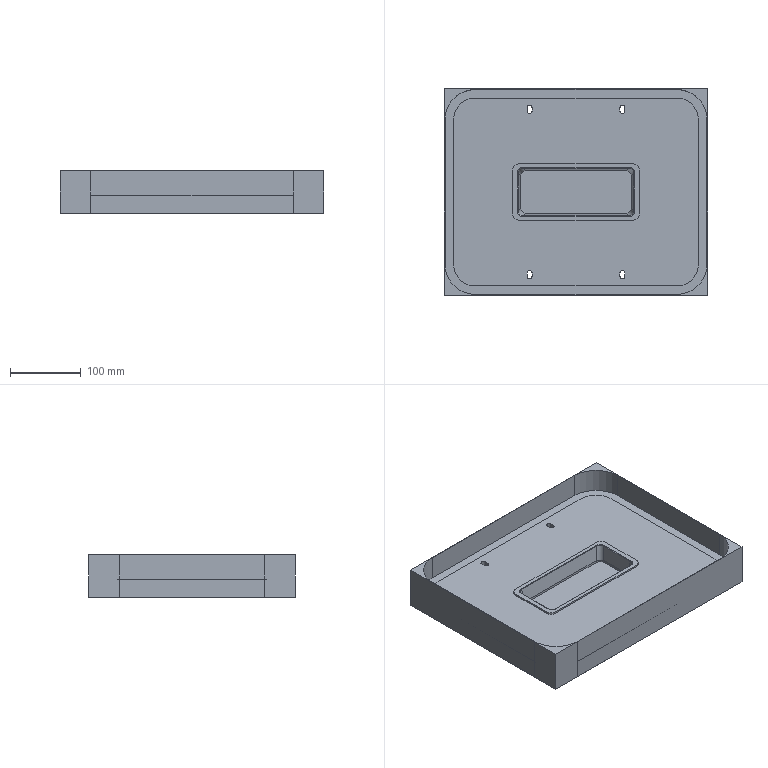CAM job | NX | 3-axis milling | part box 371 x 291 x 60.5 mm | stock box 371 x 291 x 60.5 mm
Tools:
number,name,description,diameter,corner_radius,flute_length,length,flutes
0,R1.5,Milling Tool-Ball Mill,3.0,1.5,50.0,75.0,2
0,D10,No Description,10.0,0.0,20.0,60.0,2
0,D6,No Description,6.0,0.0,0.0,35.0,2
0,D16R0.8,No Description,16.0,0.8,50.0,90.0,2
Operations:
program,operation,operation_type,tool,method,geometry_group,spindle_rpm,surface_speed,feed_per_tooth,feed_cut,feed_plunge,cut_length_mm,path_length_mm,cut_time_min,machine_time_min
A-01,CAVITY_MILL,CavityMilling,D16R0.8,METHOD,21A,8000.0,1256.0,0.2812,4500.0,100.0,898519.652,912035.959,199.671,201.023
A-02,FACE_MILLING,FaceMilling,D10,METHOD,21A,8000.0,1256.0,0.125,2000.0,100.0,13193.477,13379.477,6.597,6.615
A-03,CONTOUR_AREA,SurfaceContour,R1.5,METHOD,21A,9000.0,282.0,0.25,4500.0,100.0,57014.068,57543.112,12.67,12.723
A-03,PLANAR_TEXT,Engraving,R1.5,METHOD,21A,9000.0,84.0,0.1111,2000.0,100.0,778.501,5390.287,0.7284,1.19
A-04,PLANAR_MILL,PlanarMilling,D6,METHOD,21A,8000.0,653.0,0.25,4000.0,100.0,6198.986,7546.682,1.55,1.685
A-05,PLANAR_MILL_COPY,PlanarMilling,D10,METHOD,21A,20786.0,653.0,0.0962,4000.0,100.0,4745.738,4981.538,1.186,1.21
A-05,PLANAR_MILL_COPY_COPY,PlanarMilling,D10,METHOD,21A,20786.0,653.0,0.0962,4000.0,100.0,31911.453,32124.253,7.978,7.999